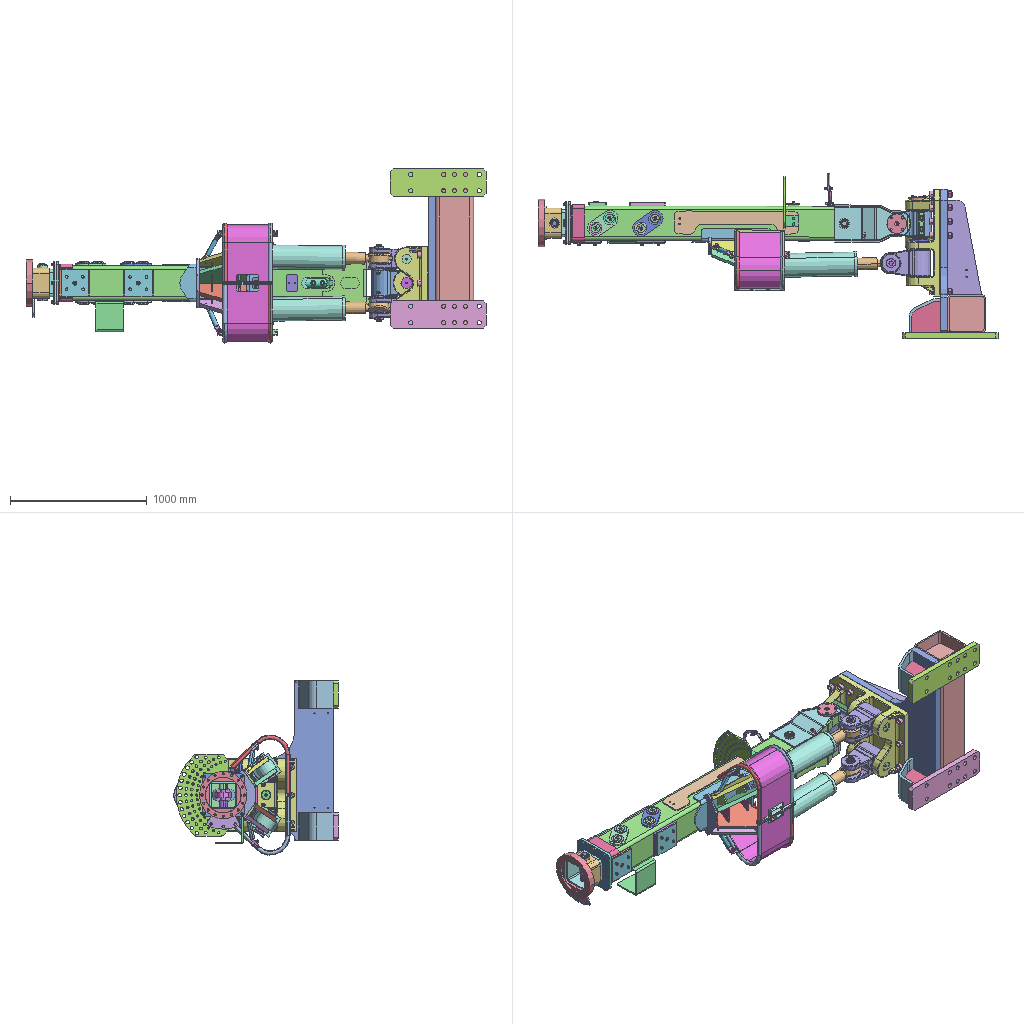Assembly | SolidWorks | 116 different items | 430 placed | box 3365 x 1207 x 1274 mm
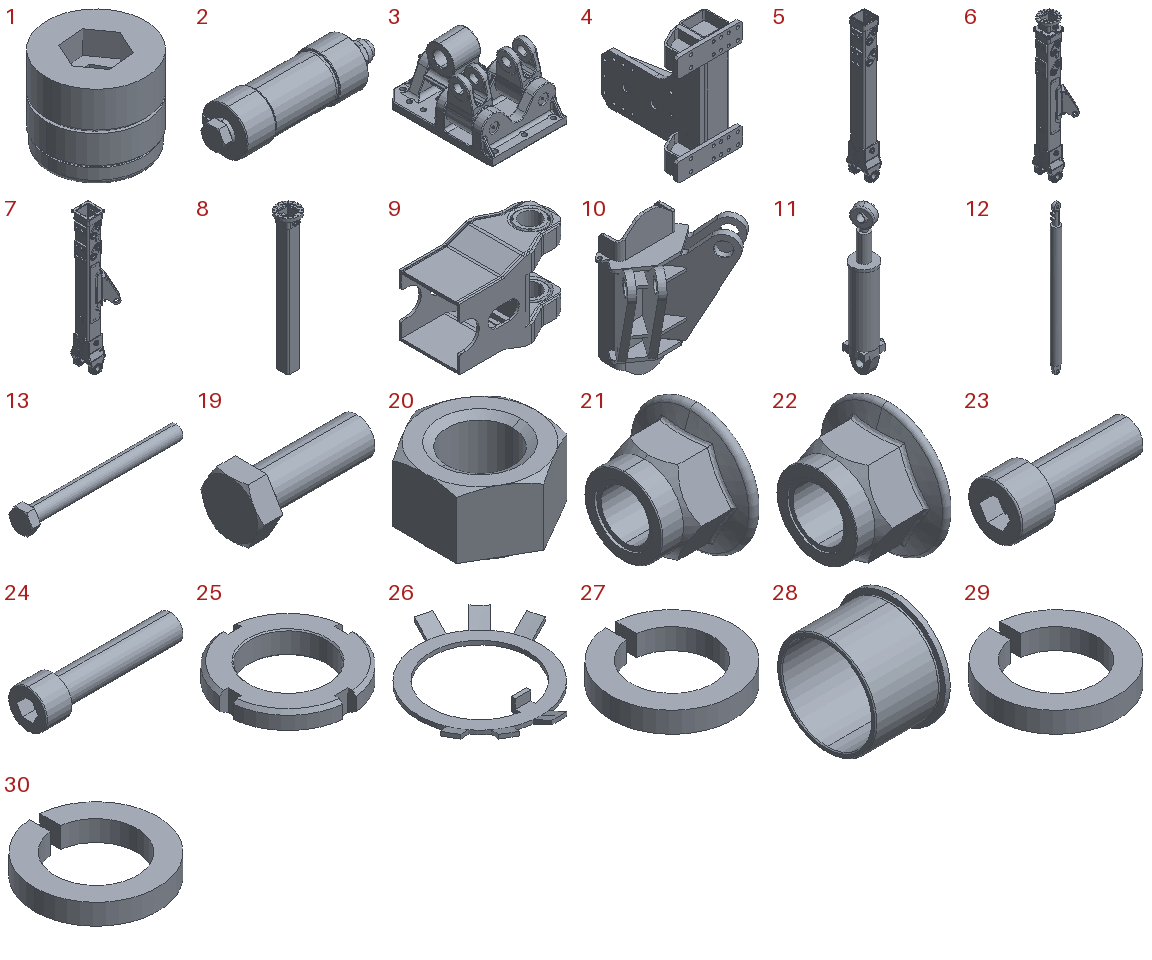Parts list (item | name | quantity | parent item | size | volume | features):
1 | (subassembly) | x14 | in 6 | 64 x 64 x 55 mm | 147055 mm3 | -
2 | (subassembly) | x4 | - | 222.5 x 65 x 65 mm | 514979 mm3 | features MirrorCompFeat 1, ReferencePattern 1
3 | (subassembly) | x1 | - | 533.36 x 780 x 459.48 mm | 60459444 mm3 | features CompositeCurve 2
4 | (subassembly) | x1 | - | 700 x 1090 x 1165 mm | 77907323 mm3 | features 3DProfileFeature 2, Cut 2, HoleWzd 2, MirrorCompFeat 2, ReferencePattern 2
5 | (subassembly) | x1 | in 7 | 291 x 352 x 2492 mm | 37081003 mm3 | features Cut 9, ReferencePattern 4, MirrorCompFeat 3, Chamfer 1, LocalLPattern 1, MirrorPattern 1, RefAxis 1
6 | (subassembly) | x1 | - | - | 96493183 mm3 | -
7 | (subassembly) | x1 | in 6 | 556.673 x 564.682 x 2503 mm | 53004232 mm3 | features MirrorCompFeat 3, ReferencePattern 3
8 | (subassembly) | x1 | in 6 | 348 x 348 x 2185 mm | 22246675 mm3 | features Cut 4, Chamfer 1, CosmeticWeldCutList 1
9 | (subassembly) | x1 | in 5 | 552.5 x 271 x 352 mm | 8203218 mm3 | features MirrorCompFeat 4, Cut 3, ReferencePattern 3, Chamfer 2, 3DProfileFeature 1, CirPattern 1, HoleWzd 1, MirrorPattern 1
10 | (subassembly) | x1 | in 7 | 564.682 x 359.673 x 650 mm | 12589036 mm3 | features ReferencePattern 8, MirrorCompFeat 6, Cut 2, Chamfer 1, LocalLPattern 1
11 | (subassembly) | x2 | - | 197.5 x 185 x 1126 mm | 10624377 mm3 | -
12 | (subassembly) | x1 | in 6 | 120 x 120 x 2210 mm | 15137402 mm3 | -
13 | - | x4 | in 2 | 222.5 x 34.641 x 30 mm | 75509 mm3 | features RevCut 3, Extrusion 1, Fillet 1, LPattern 1, Revolution 1
14 | - | x1 | in 9 | - | - | -
15 | - | x1 | in 9 | - | - | -
16 | - | x1 | in 9 | - | - | -
17 | - | x1 | in 9 | - | - | -
18 | - | x1 | in 9 | - | - | -
19 | - | x10 | in 6 | 42.5 x 20.785 x 18 mm | 6004 mm3 | features RevCut 3, Extrusion 1, Fillet 1, LPattern 1, Revolution 1
20 | - | x11 | - | 44.037 x 50.85 x 25.6 mm | 28405 mm3 | features ICE 2, RevCut 2, Extrusion 1
21 | - | x10 | - | 16.1 x 26 x 26 mm | 3234 mm3 | features Cut 2, Revolution 2, Boss 1, Chamfer 1, Fillet 1
22 | - | x4 | in 2 | 24.8 x 42.8 x 42.8 mm | 13100 mm3 | features Cut 2, Revolution 2, Boss 1, Chamfer 1, Fillet 1
23 | - | x6 | in 3 | 40 x 16 x 16 mm | 4080 mm3 | features BlendCut 1, Cut 1, Fillet 1, LPattern 1, RevCut 1, Revolution 1
24 | - | x12 | - | 170 x 45 x 45 mm | 138762 mm3 | features BlendCut 1, Cut 1, Fillet 1, LPattern 1, RevCut 1, Revolution 1
25 | - | x2 | in 6 | 54.672 x 54.672 x 10 mm | 12577 mm3 | features Chamfer 3, CirPattern 1, Cut 1, Extrusion 1
26 | - | x2 | in 6 | 56.873 x 59.449 x 5 mm | 1338 mm3 | features Boss 1, Cut 1, Revolution 1
27 | - | x8 | - | 15.372 x 15.344 x 2.6 mm | 261.313 mm3 | features Extrusion 1
28 | - | x4 | in 3 | 70 x 110 x 110 mm | 112148 mm3 | features Revolution 1
29 | - | x46 | in 3, 6 | 18.367 x 18.334 x 3.1 mm | 444.091 mm3 | features Extrusion 1
30 | - | x4 | - | 24.356 x 24.313 x 4.1 mm | 1031 mm3 | features Extrusion 1
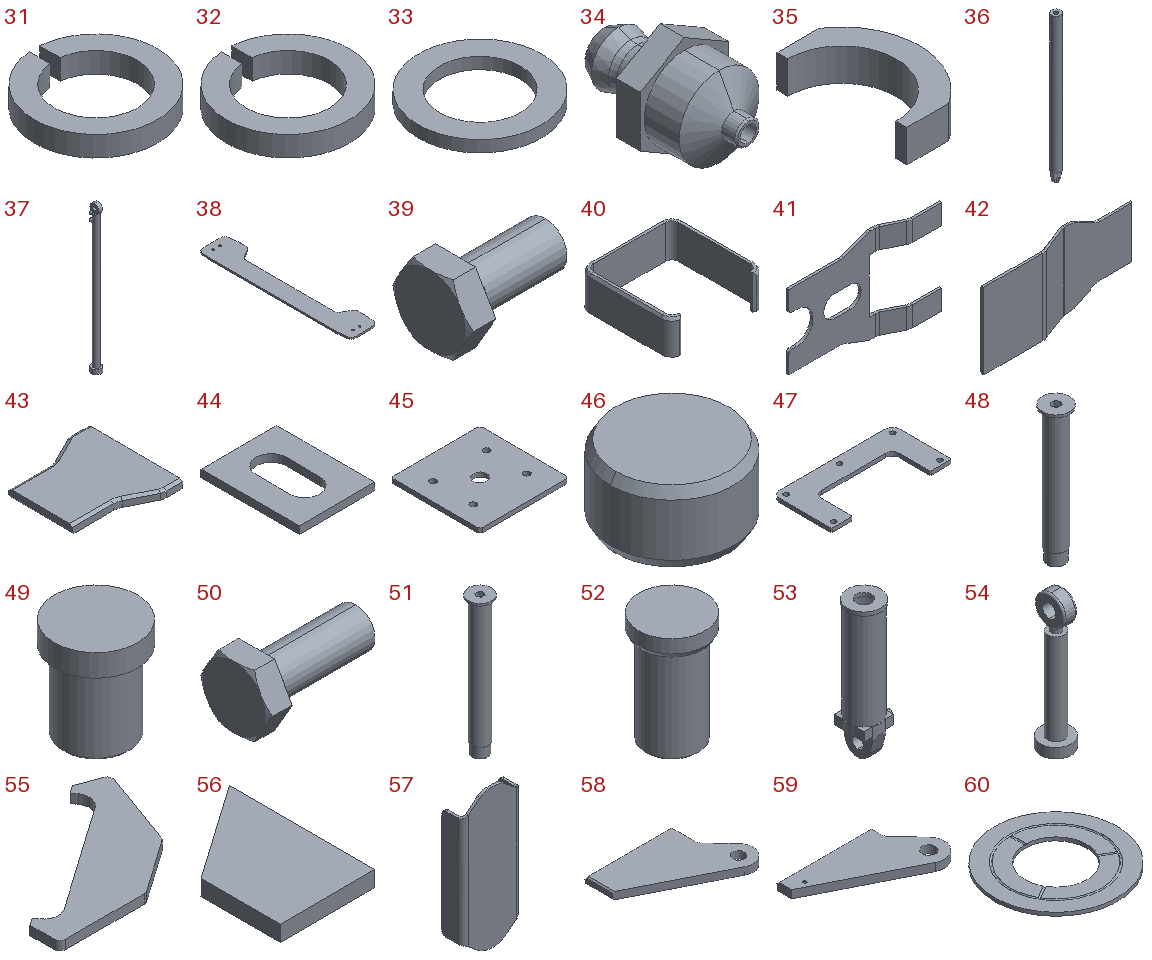31 | - | x4 | in 2 | 30.149 x 30.097 x 5 mm | 1905 mm3 | features Extrusion 1
32 | - | x11 | - | 45.424 x 45.346 x 7.5 mm | 6464 mm3 | features Extrusion 1
33 | - | x4 | in 3 | 16 x 16 x 1.5 mm | 171.708 mm3 | features Extrusion 1
34 | - | x20 | in 1, 3, 6 | 11 x 18 x 12.702 mm | 898.201 mm3 | features Boss 1, Chamfer 1, Revolution 1
35 | - | x2 | in 9 | 100 x 168 x 42 mm | 287014 mm3 | features ICE 2, Extrusion 1
36 | - | x1 | in 12 | 120 x 120 x 1920 mm | 9594518 mm3 | features ICE 4, Extrusion 1
37 | - | x1 | in 12 | 100 x 110 x 1610 mm | 5542883 mm3 | features ICE 5, Fillet 2, Extrusion 1
38 | - | x2 | in 7 | 170 x 909.794 x 10 mm | 1088199 mm3 | features 3DProfileFeature 1, Extrusion 1, HoleWzd 1
39 | - | x4 | in 3 | 26.4 x 18.475 x 16 mm | 2959 mm3 | features RevCut 3, Extrusion 1, Fillet 1, LPattern 1, Revolution 1
40 | - | x1 | in 5 | 276 x 274.941 x 100 mm | 939173 mm3 | features Chamfer 2, Extrusion 1, FlatPattern 1, RefAxis 1, SheetMetal 1, SolidToSheetMetal 1
41 | - | x2 | in 9 | 530 x 51.056 x 352 mm | 1033403 mm3 | features Fillet 3, Cut 1, Extrusion 1, FlatPattern 1, ICE 1, SheetMetal 1, SolidToSheetMetal 1
42 | - | x2 | in 9 | 530 x 50 x 251 mm | 1438713 mm3 | features Chamfer 2, Cut 1, Extrusion 1, FlatPattern 1, SheetMetal 1, SolidToSheetMetal 1
43 | - | x2 | in 9 | 250 x 251 x 20 mm | 983303 mm3 | features Chamfer 2, Extrusion 1
44 | - | x1 | in 9 | 202 x 261 x 20 mm | 809909 mm3 | features Cut 1, Extrusion 1
45 | - | x2 | in 6 | 200 x 200 x 10 mm | 386274 mm3 | features Chamfer 1, Extrusion 1, ICE 1
46 | - | x2 | in 9 | 130 x 130 x 75 mm | 972611 mm3 | features Chamfer 1, Extrusion 1
47 | - | x2 | in 6 | 310 x 152.5 x 10 mm | 269228 mm3 | features Chamfer 1, Extrusion 1, ICE 1
48 | - | x1 | in 6 | 55 x 55 x 275 mm | 342139 mm3 | features ICE 4, Chamfer 2, Fillet 2, Extrusion 1
49 | - | x2 | in 8 | 75 x 75 x 90 mm | 285538 mm3 | features Chamfer 1, Extrusion 1, ICE 1, RefAxis 1, RevCut 1
50 | - | x8 | - | 31.4 x 18.475 x 16 mm | 3352 mm3 | features RevCut 3, Extrusion 1, Fillet 1, LPattern 1, Revolution 1
51 | - | x1 | in 6 | 55 x 55 x 330 mm | 411254 mm3 | features ICE 4, Chamfer 2, Fillet 2, Extrusion 1
52 | - | x2 | in 5 | 75 x 75 x 125 mm | 382842 mm3 | features Chamfer 2, Extrusion 1, ICE 1, RefAxis 1, RevCut 1
53 | - | x2 | in 11 | 197.5 x 185 x 748 mm | 5801023 mm3 | features ICE 6, Extrusion 1
54 | - | x2 | in 11 | 155 x 155 x 685 mm | 4561292 mm3 | features ICE 3, Extrusion 1, Fillet 1, RevCut 1
55 | - | x2 | in 10 | 296.858 x 227.831 x 16 mm | 414208 mm3 | features Extrusion 1, Fillet 1
56 | - | x4 | in 10 | 72 x 110.415 x 12 mm | 73619 mm3 | features Extrusion 1
57 | - | x1 | in 10 | 274 x 100 x 650 mm | 2917891 mm3 | features Fillet 3, Extrusion 1, FlatPattern 1, ICE 1, SheetMetal 1, SolidToSheetMetal 1
58 | - | x1 | in 10 | 450 x 310 x 30 mm | 2452463 mm3 | features ICE 2, Chamfer 1, Extrusion 1, Fillet 1
59 | - | x1 | in 10 | 450 x 245.418 x 30 mm | 1807994 mm3 | features Chamfer 2, 3DProfileFeature 1, Extrusion 1, Fillet 1, HoleWzd 1, ICE 1
60 | - | x4 | in 3 | 180 x 180 x 5 mm | 93702 mm3 | features CirPattern 1, Extrusion 1, ICE 1, SweepCut 1
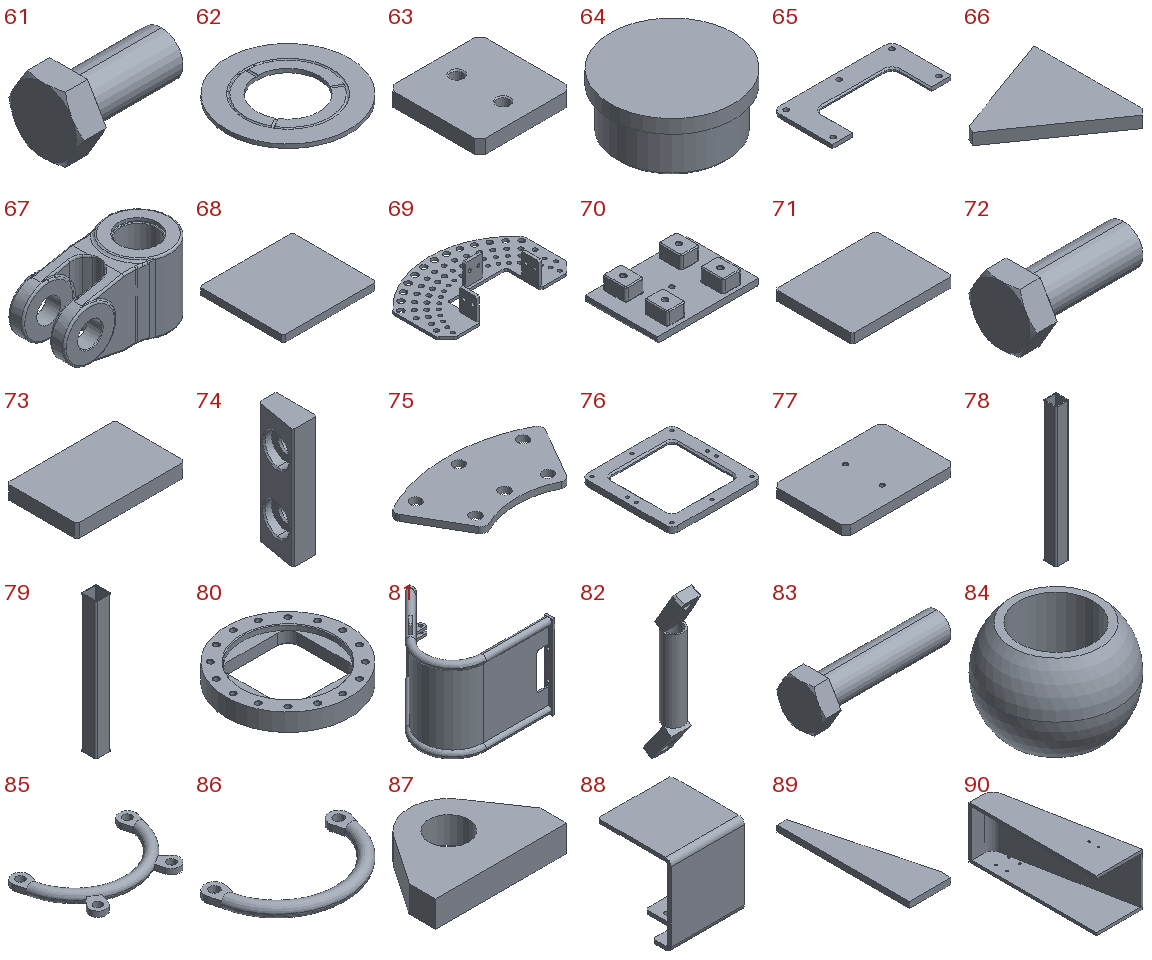61 | - | x10 | - | 32.5 x 20.785 x 18 mm | 4896 mm3 | features RevCut 3, Extrusion 1, Fillet 1, LPattern 1, Revolution 1
62 | - | x4 | in 3 | 160 x 160 x 5 mm | 73404 mm3 | features CirPattern 1, Extrusion 1, ICE 1, SweepCut 1
63 | - | x2 | in 7 | 80 x 80 x 12 mm | 74210 mm3 | features 3DProfileFeature 1, Chamfer 1, Extrusion 1, HoleWzd 1
64 | - | x8 | in 5 | 90 x 90 x 40 mm | 213919 mm3 | features Chamfer 1, Extrusion 1, ICE 1
65 | - | x2 | in 6 | 310 x 155 x 10 mm | 271244 mm3 | features Chamfer 2, Extrusion 1, ICE 1
66 | - | x2 | in 10 | 109.653 x 118.533 x 12 mm | 84519 mm3 | features Chamfer 1, Extrusion 1
67 | - | x2 | in 3 | 360 x 170 x 190 mm | 5382355 mm3 | features Fillet 14, ICE 11, Chamfer 4, MirrorPattern 2, Extrusion 1
68 | - | x2 | in 5 | 220 x 200 x 16 mm | 703200 mm3 | features Chamfer 1, Extrusion 1
69 | - | x1 | - | 600 x 380 x 112 mm | 1912190 mm3 | features ICE 7, Chamfer 4, Fillet 2, Extrusion 1
70 | - | x2 | in 6 | 220 x 156 x 41 mm | 648934 mm3 | features Fillet 4, ICE 3, 3DProfileFeature 2, HoleWzd 2, Chamfer 1, Extrusion 1
71 | - | x1 | in 5 | 260 x 200 x 25 mm | 1298750 mm3 | features Chamfer 1, Extrusion 1
72 | - | x8 | in 6 | 37.5 x 20.785 x 18 mm | 5461 mm3 | features RevCut 3, Extrusion 1, Fillet 1, LPattern 1, Revolution 1
73 | - | x1 | in 5 | 200 x 130 x 25 mm | 648750 mm3 | features Chamfer 1, Extrusion 1
74 | - | x2 | - | 31.677 x 55 x 160 mm | 198340 mm3 | features Chamfer 2, ICE 2, Extrusion 1
75 | - | x1 | - | 242.471 x 129.725 x 10 mm | 215713 mm3 | features Extrusion 1, Fillet 1, ICE 1
76 | - | x1 | in 7 | 310 x 310 x 20 mm | 773843 mm3 | features 3DProfileFeature 1, Chamfer 1, Extrusion 1, Fillet 1, HoleWzd 1, ICE 1
77 | - | x2 | in 7 | 120 x 80 x 10 mm | 95220 mm3 | features 3DProfileFeature 1, Chamfer 1, Extrusion 1, HoleWzd 1
78 | - | x1 | in 8 | 200 x 200 x 2150 mm | 18654812 mm3 | features Extrusion 1, Fillet 1, ICE 1
79 | - | x1 | in 5 | 250 x 250 x 2220 mm | 24230431 mm3 | features Chamfer 1, Extrusion 1, ICE 1, RefAxis 1
80 | - | x1 | in 8 | 348 x 348 x 50 mm | 2451722 mm3 | features Chamfer 2, ICE 2, 3DProfileFeature 1, CirPattern 1, Extrusion 1, HoleWzd 1
81 | - | x2 | - | 439 x 443.772 x 444 mm | 2517725 mm3 | features ICE 9, Chamfer 5, Sweep 2, BossThin 1
82 | - | x2 | - | 32 x 64.415 x 248.288 mm | 82986 mm3 | features ICE 4, Chamfer 2, Extrusion 1
83 | - | x18 | in 3 | 57.5 x 20.785 x 18 mm | 7723 mm3 | features RevCut 3, Extrusion 1, Fillet 1, LPattern 1, Revolution 1
84 | - | x2 | in 11 | 100 x 100 x 70 mm | 262061 mm3 | features ICE 2, Revolution 1
85 | - | x1 | - | 225.916 x 141.102 x 20 mm | 58505 mm3 | features ICE 3, MirrorPattern 1, Sweep 1
86 | - | x1 | - | 225.916 x 125 x 20 mm | 44773 mm3 | features ICE 2, MirrorPattern 1, Sweep 1
87 | - | x6 | in 7, 10 | 50 x 35 x 10 mm | 11273 mm3 | features Extrusion 1
88 | - | x1 | - | 200 x 200 x 220 mm | 944720 mm3 | features ICE 4, Fillet 3, Chamfer 1, Extrusion 1, FlatPattern 1, SheetMetal 1, SolidToSheetMetal 1
89 | - | x1 | in 4 | 210 x 670 x 30 mm | 2733000 mm3 | features Extrusion 1
90 | - | x1 | in 4 | 250 x 690 x 280 mm | 6785212 mm3 | features 3DProfileFeature 2, HoleWzd 2, ICE 2, Extrusion 1
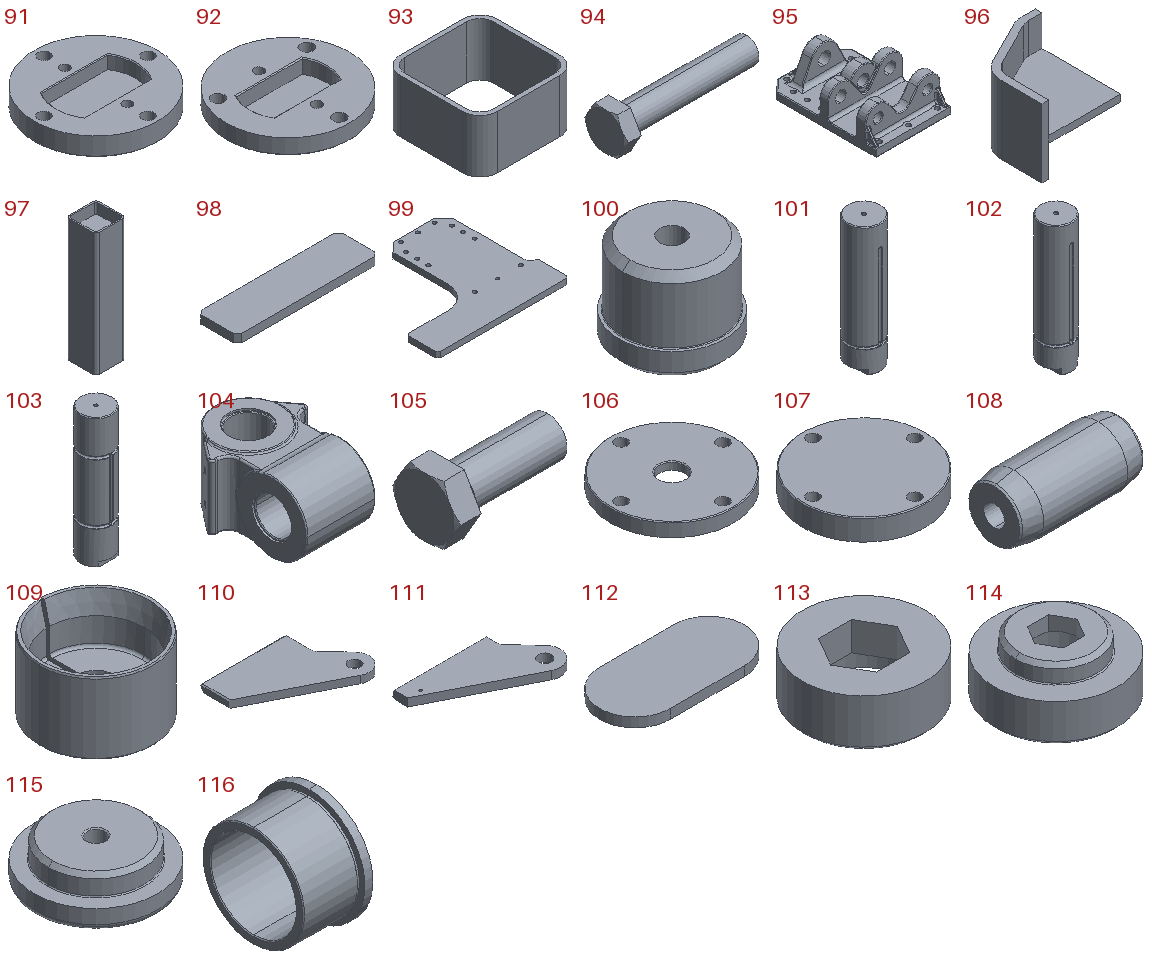91 | - | x1 | in 3 | 148 x 148 x 25 mm | 305929 mm3 | features Chamfer 3, ICE 3, 3DProfileFeature 1, Extrusion 1, HoleWzd 1
92 | - | x2 | in 3 | 138 x 138 x 20 mm | 204024 mm3 | features Chamfer 3, ICE 3, 3DProfileFeature 1, Extrusion 1, HoleWzd 1
93 | - | x1 | in 8 | 220 x 220 x 120 mm | 935894 mm3 | features Extrusion 1
94 | - | x2 | - | 67.5 x 20.785 x 18 mm | 8854 mm3 | features RevCut 3, Extrusion 1, Fillet 1, LPattern 1, Revolution 1
95 | - | x1 | in 3 | 530 x 780 x 260 mm | 33233633 mm3 | features Fillet 26, ICE 14, Chamfer 4, MirrorPattern 3, 3DProfileFeature 2, HoleWzd 2, LPattern 2, Extrusion 1
96 | - | x2 | in 4 | 230 x 250 x 200 mm | 2385457 mm3 | features Extrusion 1, ICE 1
97 | - | x1 | in 4 | 280 x 280 x 1165 mm | 17020849 mm3 | features ICE 2, Extrusion 1, MirrorPattern 1
98 | - | x2 | in 4 | 700 x 200 x 40 mm | 5568000 mm3 | features Chamfer 1, Extrusion 1
99 | - | x1 | in 4 | 1165 x 1050 x 50 mm | 36177793 mm3 | features Chamfer 3, ICE 2, 3DProfileFeature 1, Extrusion 1, HoleWzd 1
100 | - | x2 | in 3 | 75 x 75 x 63 mm | 232128 mm3 | features 3DProfileFeature 1, Chamfer 1, Extrusion 1, Fillet 1, HoleWzd 1, ICE 1
101 | - | x1 | in 3 | 90 x 90 x 350 mm | 2147115 mm3 | features Fillet 5, ICE 5, 3DProfileFeature 3, HoleWzd 3, Chamfer 2, RevCut 2, Extrusion 1, MirrorPattern 1, RefAxis 1
102 | - | x2 | in 3 | 80 x 80 x 330 mm | 1584103 mm3 | features ICE 5, Fillet 4, 3DProfileFeature 3, HoleWzd 3, Chamfer 2, RevCut 2, Extrusion 1, MirrorPattern 1, RefAxis 1
103 | - | x1 | - | 90 x 90 x 372 mm | 2295512 mm3 | features Fillet 5, ICE 5, 3DProfileFeature 2, HoleWzd 2, MirrorPattern 2, RevCut 2, Chamfer 1, Extrusion 1, RefAxis 1
104 | - | x1 | in 3 | 269.383 x 350 x 195 mm | 8603541 mm3 | features Fillet 12, ICE 10, MirrorPattern 3, Chamfer 2, 3DProfileFeature 1, Extrusion 1, HoleWzd 1
105 | - | x4 | - | 50 x 27.713 x 24 mm | 12952 mm3 | features RevCut 3, Extrusion 1, Fillet 1, LPattern 1, Revolution 1
106 | - | x1 | - | 145 x 145 x 16 mm | 201040 mm3 | features ICE 3, Chamfer 1, Extrusion 1
107 | - | x1 | - | 145 x 145 x 25 mm | 302931 mm3 | features Chamfer 2, ICE 2, Extrusion 1
108 | - | x4 | in 2 | 125 x 60 x 60 mm | 297103 mm3 | features 3DProfileFeature 1, Chamfer 1, HoleWzd 1, ICE 1, Revolution 1
109 | - | x8 | in 2 | 65 x 64.985 x 41.25 mm | 63691 mm3 | features Chamfer 2, ICE 2, 3DProfileFeature 1, Extrusion 1, Fillet 1, HoleWzd 1, RevCut 1
110 | - | x1 | in 10 | 450 x 310 x 30 mm | 2452463 mm3 | features MirrorStock 1
111 | - | x1 | in 10 | 450 x 245.418 x 30 mm | 1807994 mm3 | features MirrorStock 1
112 | - | x4 | in 5 | 245 x 120 x 16 mm | 420956 mm3 | features Extrusion 1
113 | - | x14 | in 1 | 64 x 64 x 25 mm | 53818 mm3 | features ICE 2, Chamfer 1, Extrusion 1
114 | - | x14 | in 1 | 64 x 64 x 29 mm | 46539 mm3 | features Chamfer 2, ICE 2, 3DProfileFeature 1, Extrusion 1, Fillet 1, HoleWzd 1
115 | - | x14 | in 1 | 62 x 62 x 20 mm | 45800 mm3 | features ICE 3, Fillet 2, 3DProfileFeature 1, Chamfer 1, Extrusion 1, HoleWzd 1
116 | - | x4 | in 3 | 60 x 105 x 105 mm | 135111 mm3 | features Revolution 1
Mates (type | each side: item.copy, entity, surface, feature), first 394 of 672 lines:
In the top assembly
Concentric | 103.1 face cylinder Boss-Extrude 1 | assembly face
Concentric | 103.1 face cylinder M10 Tapped Hole 1 | assembly face
Coincident | 103.1 face plane Boss-Extrude 1 | assembly face
Parallel | 103.1 face plane Cut-Extrude 4 | 107.1 face plane Cut-Extrude 2 | 2 times
Concentric | 103.1 face cylinder Boss-Extrude 1 | 60.1 face cylinder Boss-Extrude 1
Concentric | 103.1 face cylinder Boss-Extrude 1 | 60.2 face cylinder Boss-Extrude 1
Concentric | 28.1 face cylinder Revolve 1 | 103.1 face cylinder Boss-Extrude 1
Concentric | 103.1 face cylinder Boss-Extrude 1 | 106.1 face cylinder Boss-Extrude 1
Coincident | 99.1 face plane | 32.1 face plane Extrude 1
Coincident | 20.1 face plane Boss-Extrude 1 | 32.1 face plane Extrude 1
Concentric | 20.1 face cylinder Boss-Extrude 1 | 24.1 face cylinder Base-Revolve
Concentric | 32.1 face cylinder Extrude 1 | 24.1 face cylinder Base-Revolve
Coincident | 20.2 face plane Boss-Extrude 1 | 32.2 face plane Extrude 1
Concentric | 24.2 face cylinder Base-Revolve | 20.2 face cylinder Boss-Extrude 1
Concentric | 24.2 face cylinder Base-Revolve | 32.2 face cylinder Extrude 1
Coincident | 99.1 face plane | 32.2 face plane Extrude 1
Coincident | 20.3 face plane Boss-Extrude 1 | 32.3 face plane Extrude 1
Concentric | 24.3 face cylinder Base-Revolve | 20.3 face cylinder Boss-Extrude 1
Concentric | 24.3 face cylinder Base-Revolve | 32.3 face cylinder Extrude 1
Coincident | 99.1 face plane | 32.3 face plane Extrude 1
Coincident | 20.4 face plane Boss-Extrude 1 | 32.4 face plane Extrude 1
Concentric | 24.4 face cylinder Base-Revolve | 20.4 face cylinder Boss-Extrude 1
Concentric | 24.4 face cylinder Base-Revolve | 32.4 face cylinder Extrude 1
Coincident | 99.1 face plane | 32.4 face plane Extrude 1
Coincident | 20.5 face plane Boss-Extrude 1 | 32.5 face plane Extrude 1
Concentric | 24.5 face cylinder Base-Revolve | 20.5 face cylinder Boss-Extrude 1
Concentric | 24.5 face cylinder Base-Revolve | 32.5 face cylinder Extrude 1
Coincident | 99.1 face plane | 32.5 face plane Extrude 1
Coincident | 20.6 face plane Boss-Extrude 1 | 32.6 face plane Extrude 1
Concentric | 24.6 face cylinder Base-Revolve | 20.6 face cylinder Boss-Extrude 1
Concentric | 24.6 face cylinder Base-Revolve | 32.6 face cylinder Extrude 1
Coincident | 99.1 face plane | 32.6 face plane Extrude 1
Coincident | 20.7 face plane Boss-Extrude 1 | 32.7 face plane Extrude 1
Concentric | 24.7 face cylinder Base-Revolve | 20.7 face cylinder Boss-Extrude 1
Concentric | 24.7 face cylinder Base-Revolve | 32.7 face cylinder Extrude 1
Coincident | 99.1 face plane | 32.7 face plane Extrude 1
Concentric | 107.1 face cylinder Cut-Extrude 1 | 27.1 face cylinder Extrude 1
Coincident | 107.1 face plane Boss-Extrude 1 | 27.1 face plane Extrude 1
Concentric | 50.1 face cylinder Boss-Revolve 1 | 27.1 face cylinder Extrude 1
Coincident | 50.1 face plane Base-Extrude | 27.1 face plane Extrude 1
Coincident | 103.1 face plane Boss-Extrude 1 | 107.1 face plane Cut-Extrude 2
Concentric | 103.1 face cylinder Boss-Extrude 1 | 107.1 face cylinder Boss-Extrude 1
Coincident | 81.1 face plane Boss-Extrude 5 | 81.2 face plane Boss-Extrude 5
Concentric | 81.1 face cylinder Cut-Extrude 5 | 81.2 face cylinder Cut-Extrude 5
Concentric | 81.2 face cylinder Boss-Extrude 6 | 82.1 face cylinder Cut-Extrude 2
Coincident | 81.2 face plane Boss-Extrude 6 | 82.1 face plane Boss-Extrude 3
Concentric | 85.1 face cylinder Boss-Extrude 1 | 86.1 face cylinder Boss-Extrude 1
Concentric | 85.1 face cylinder Mirror 1 | 86.1 face cylinder Mirror 1
Coincident | 85.1 face plane Mirror 1 | 86.1 face plane Mirror 1
Concentric | 81.1 face cylinder Boss-Extrude 6 | 82.2 face cylinder Cut-Extrude 2
Coincident | 81.1 face plane Boss-Extrude 6 | 82.2 face plane Boss-Extrude 3
Concentric | 105.1 face cylinder Boss-Revolve 1 | 30.1 face cylinder Extrude 1
Coincident | 105.1 face plane Base-Extrude | 30.1 face plane Extrude 1
Concentric | 74.1 face cylinder Cut-Extrude 3 | 105.1 face cylinder Boss-Revolve 1
Coincident | 74.1 face plane Cut-Extrude 2 | 30.1 face plane Extrude 1
Concentric | 105.2 face cylinder Boss-Revolve 1 | 30.2 face cylinder Extrude 1
Coincident | 105.2 face plane Base-Extrude | 30.2 face plane Extrude 1
Concentric | 74.1 face cylinder Cut-Extrude 3 | 105.2 face cylinder Boss-Revolve 1
Coincident | 74.1 face plane Cut-Extrude 2 | 30.2 face plane Extrude 1
Concentric | 105.3 face cylinder Boss-Revolve 1 | 30.3 face cylinder Extrude 1
Coincident | 105.3 face plane Base-Extrude | 30.3 face plane Extrude 1
Concentric | 74.2 face cylinder Cut-Extrude 3 | 105.3 face cylinder Boss-Revolve 1
Coincident | 74.2 face plane Cut-Extrude 2 | 30.3 face plane Extrude 1
Concentric | 105.4 face cylinder Boss-Revolve 1 | 30.4 face cylinder Extrude 1
Coincident | 105.4 face plane Base-Extrude | 30.4 face plane Extrude 1
Concentric | 74.2 face cylinder Cut-Extrude 3 | 105.4 face cylinder Boss-Revolve 1
Coincident | 74.2 face plane Cut-Extrude 2 | 30.4 face plane Extrude 1
Concentric | 50.2 face cylinder Boss-Revolve 1 | 27.2 face cylinder Extrude 1
Coincident | 50.2 face plane Base-Extrude | 27.2 face plane Extrude 1
Concentric | 107.1 face cylinder Cut-Extrude 1 | 27.2 face cylinder Extrude 1
Coincident | 107.1 face plane Boss-Extrude 1 | 27.2 face plane Extrude 1
Concentric | 50.3 face cylinder Boss-Revolve 1 | 27.3 face cylinder Extrude 1
Coincident | 50.3 face plane Base-Extrude | 27.3 face plane Extrude 1
Concentric | 107.1 face cylinder Cut-Extrude 1 | 27.3 face cylinder Extrude 1
Coincident | 107.1 face plane Boss-Extrude 1 | 27.3 face plane Extrude 1
Concentric | 50.4 face cylinder Boss-Revolve 1 | 27.4 face cylinder Extrude 1
Coincident | 50.4 face plane Base-Extrude | 27.4 face plane Extrude 1
Concentric | 107.1 face cylinder Cut-Extrude 1 | 27.4 face cylinder Extrude 1
Coincident | 107.1 face plane Boss-Extrude 1 | 27.4 face plane Extrude 1
Concentric | 50.5 face cylinder Boss-Revolve 1 | 27.5 face cylinder Extrude 1
Coincident | 50.5 face plane Base-Extrude | 27.5 face plane Extrude 1
Concentric | 106.1 face cylinder Cut-Extrude 1 | 27.5 face cylinder Extrude 1
Coincident | 106.1 face plane Boss-Extrude 1 | 27.5 face plane Extrude 1
Concentric | 50.6 face cylinder Boss-Revolve 1 | 27.6 face cylinder Extrude 1
Coincident | 50.6 face plane Base-Extrude | 27.6 face plane Extrude 1
Concentric | 106.1 face cylinder Cut-Extrude 1 | 27.6 face cylinder Extrude 1
Coincident | 106.1 face plane Boss-Extrude 1 | 27.6 face plane Extrude 1
Concentric | 50.7 face cylinder Boss-Revolve 1 | 27.7 face cylinder Extrude 1
Coincident | 50.7 face plane Base-Extrude | 27.7 face plane Extrude 1
Concentric | 106.1 face cylinder Cut-Extrude 1 | 27.7 face cylinder Extrude 1
Coincident | 106.1 face plane Boss-Extrude 1 | 27.7 face plane Extrude 1
Concentric | 50.8 face cylinder Boss-Revolve 1 | 27.8 face cylinder Extrude 1
Coincident | 50.8 face plane Base-Extrude | 27.8 face plane Extrude 1
Coincident | 106.1 face plane Boss-Extrude 1 | 27.8 face plane Extrude 1
Concentric | 106.1 face cylinder Cut-Extrude 1 | 50.8 face cylinder Boss-Revolve 1
Coincident | 103.1 face plane Cut-Extrude 7 | 33.1 face plane Extrude 1
Concentric | 103.1 face cylinder M10 Tapped Hole 2 | 33.1 face cylinder Extrude 1
Coincident | 39.1 face plane Base-Extrude | 33.1 face plane Extrude 1
Concentric | 103.1 face cylinder M10 Tapped Hole 2 | 39.1 face cylinder Boss-Revolve 1
Concentric | 103.1 face cylinder M10 Tapped Hole 1 | 34.1 face cylinder Revolve 2
Coincident | 103.1 face plane Boss-Extrude 1 | 34.1 face plane Revolve 2
Concentric | 83.1 face cylinder Boss-Revolve 1 | 21.1 face cylinder Cut-Extrude 3
Coincident | 85.1 face plane Boss-Extrude 2 | 21.1 face plane Base-Revolve
Concentric | 83.1 face cylinder Boss-Revolve 1 | 29.1 face cylinder Extrude 1
Coincident | 83.1 face plane Base-Extrude | 29.1 face plane Extrude 1
Concentric | 83.2 face cylinder Boss-Revolve 1 | 21.2 face cylinder Cut-Extrude 3
Concentric | 83.2 face cylinder Boss-Revolve 1 | 29.2 face cylinder Extrude 1
Coincident | 83.2 face plane Base-Extrude | 29.2 face plane Extrude 1
Concentric | 85.1 face cylinder Boss-Extrude 2 | 83.2 face cylinder Boss-Revolve 1
Coincident | 85.1 face plane Boss-Extrude 2 | 21.2 face plane Base-Revolve
Concentric | 83.3 face cylinder Boss-Revolve 1 | 21.3 face cylinder Cut-Extrude 3
Concentric | 83.3 face cylinder Boss-Revolve 1 | 29.3 face cylinder Extrude 1
Coincident | 83.3 face plane Base-Extrude | 29.3 face plane Extrude 1
Concentric | 85.1 face cylinder Mirror 1 | 83.3 face cylinder Boss-Revolve 1
Coincident | 86.1 face plane Mirror 1 | 21.3 face plane Base-Revolve
Coincident | 85.1 face plane Mirror 1 | 29.3 face plane Extrude 1
Concentric | 83.4 face cylinder Boss-Revolve 1 | 21.4 face cylinder Cut-Extrude 3
Concentric | 83.4 face cylinder Boss-Revolve 1 | 29.4 face cylinder Extrude 1
Coincident | 83.4 face plane Base-Extrude | 29.4 face plane Extrude 1
Concentric | 85.1 face cylinder Boss-Extrude 1 | 83.4 face cylinder Boss-Revolve 1
Coincident | 86.1 face plane Boss-Extrude 1 | 21.4 face plane Base-Revolve
Coincident | 85.1 face plane Boss-Extrude 1 | 29.4 face plane Extrude 1
Coincident | 81.2 face plane Boss-Extrude 5 | 21.5 face plane Base-Revolve
Concentric | 81.2 face cylinder Cut-Extrude 6 | 21.5 face cylinder Cut-Extrude 3
Concentric | 69.1 face cylinder Cut-Extrude 1 | 29.5 face cylinder Extrude 1
Concentric | 69.1 face cylinder Cut-Extrude 1 | 61.1 face cylinder Boss-Revolve 1
Coincident | 61.1 face plane Base-Extrude | 29.5 face plane Extrude 1
Coincident | 69.1 face plane Boss-Extrude 2 | 29.5 face plane Extrude 1
Coincident | 29.6 face plane Extrude 1 | 61.2 face plane Base-Extrude
Concentric | 69.1 face cylinder Cut-Extrude 1 | 29.6 face cylinder Extrude 1
Concentric | 69.1 face cylinder Cut-Extrude 1 | 61.2 face cylinder Boss-Revolve 1
Coincident | 69.1 face plane Boss-Extrude 2 | 29.6 face plane Extrude 1
Coincident | 29.7 face plane Extrude 1 | 61.3 face plane Base-Extrude
Concentric | 69.1 face cylinder Cut-Extrude 2 | 29.7 face cylinder Extrude 1
Concentric | 69.1 face cylinder Cut-Extrude 2 | 61.3 face cylinder Boss-Revolve 1
Coincident | 69.1 face plane Boss-Extrude 2 | 29.7 face plane Extrude 1
Coincident | 29.8 face plane Extrude 1 | 61.4 face plane Base-Extrude
Concentric | 69.1 face cylinder Cut-Extrude 2 | 29.8 face cylinder Extrude 1
Concentric | 69.1 face cylinder Cut-Extrude 2 | 61.4 face cylinder Boss-Revolve 1
Coincident | 69.1 face plane Boss-Extrude 2 | 29.8 face plane Extrude 1
Coincident | 29.9 face plane Extrude 1 | 61.5 face plane Base-Extrude
Concentric | 69.1 face cylinder Cut-Extrude 1 | 29.9 face cylinder Extrude 1
Coincident | 69.1 face plane Boss-Extrude 2 | 29.9 face plane Extrude 1
Concentric | 69.1 face cylinder Cut-Extrude 1 | 61.5 face cylinder Boss-Revolve 1
Coincident | 29.10 face plane Extrude 1 | 61.6 face plane Base-Extrude
Concentric | 69.1 face cylinder Cut-Extrude 1 | 29.10 face cylinder Extrude 1
Coincident | 69.1 face plane Boss-Extrude 2 | 29.10 face plane Extrude 1
Concentric | 69.1 face cylinder Cut-Extrude 1 | 61.6 face cylinder Boss-Revolve 1
Coincident | 61.7 face plane Base-Extrude | 29.11 face plane Extrude 1
Concentric | 88.1 face cylinder 转换Body 1 | 29.11 face cylinder Extrude 1
Coincident | 88.1 face plane 转换Body 1 | 29.11 face plane Extrude 1
Concentric | 88.1 face cylinder 转换Body 1 | 61.7 face cylinder Boss-Revolve 1
Coincident | 61.8 face plane Base-Extrude | 29.12 face plane Extrude 1
Concentric | 88.1 face cylinder 转换Body 1 | 29.12 face cylinder Extrude 1
Coincident | 88.1 face plane 转换Body 1 | 29.12 face plane Extrude 1
Concentric | 88.1 face cylinder 转换Body 1 | 61.8 face cylinder Boss-Revolve 1
Concentric | 81.2 face cylinder Cut-Extrude 6 | 94.1 face cylinder Boss-Revolve 1
Coincident | 81.2 face plane Boss-Extrude 5 | 94.1 face plane Base-Extrude
Coincident | 81.1 face plane Boss-Extrude 5 | 21.6 face plane Base-Revolve
Concentric | 81.1 face cylinder Cut-Extrude 6 | 21.6 face cylinder Cut-Extrude 3
Concentric | 81.1 face cylinder Cut-Extrude 6 | 94.2 face cylinder Boss-Revolve 1
Coincident | 81.1 face plane Boss-Extrude 5 | 94.2 face plane Base-Extrude
Concentric | 21.7 face cylinder Cut-Extrude 3 | 83.5 face cylinder Boss-Revolve 1
Concentric | 83.5 face cylinder Boss-Revolve 1 | 29.13 face cylinder Extrude 1
Coincident | 83.5 face plane Base-Extrude | 29.13 face plane Extrude 1
Concentric | 81.2 face cylinder Boss-Extrude 6 | 83.5 face cylinder Boss-Revolve 1
Coincident | 82.1 face plane Boss-Extrude 3 | 21.7 face plane Base-Revolve
Coincident | 81.2 face plane Boss-Extrude 6 | 29.13 face plane Extrude 1
Concentric | 21.8 face cylinder Cut-Extrude 3 | 83.6 face cylinder Boss-Revolve 1
Concentric | 83.6 face cylinder Boss-Revolve 1 | 29.14 face cylinder Extrude 1
Coincident | 83.6 face plane Base-Extrude | 29.14 face plane Extrude 1
Concentric | 81.1 face cylinder Boss-Extrude 6 | 83.6 face cylinder Boss-Revolve 1
Coincident | 82.2 face plane Boss-Extrude 3 | 21.8 face plane Base-Revolve
Coincident | 81.1 face plane Boss-Extrude 6 | 29.14 face plane Extrude 1
Coincident | 61.9 face plane Base-Extrude | 29.15 face plane Extrude 1
Concentric | 82.2 face cylinder Cut-Extrude 1 | 29.15 face cylinder Extrude 1
Coincident | 82.2 face plane Boss-Extrude 2 | 29.15 face plane Extrude 1
Concentric | 82.2 face cylinder Cut-Extrude 1 | 61.9 face cylinder Boss-Revolve 1
Coincident | 61.10 face plane Base-Extrude | 29.16 face plane Extrude 1
Concentric | 82.1 face cylinder Cut-Extrude 1 | 29.16 face cylinder Extrude 1
Coincident | 82.1 face plane Boss-Extrude 2 | 29.16 face plane Extrude 1
Concentric | 82.1 face cylinder Cut-Extrude 1 | 61.10 face cylinder Boss-Revolve 1
Concentric | 83.7 face cylinder Boss-Revolve 1 | 21.9 face cylinder Cut-Extrude 3
Concentric | 83.7 face cylinder Boss-Revolve 1 | 29.17 face cylinder Extrude 1
Coincident | 83.7 face plane Base-Extrude | 29.17 face plane Extrude 1
Concentric | 81.1 face cylinder Cut-Extrude 5 | 83.7 face cylinder Boss-Revolve 1
Coincident | 81.1 face plane Boss-Extrude 4 | 21.9 face plane Base-Revolve
Coincident | 81.2 face plane Boss-Extrude 4 | 29.17 face plane Extrude 1
Concentric | 83.8 face cylinder Boss-Revolve 1 | 21.10 face cylinder Cut-Extrude 3
Concentric | 83.8 face cylinder Boss-Revolve 1 | 29.18 face cylinder Extrude 1
Coincident | 83.8 face plane Base-Extrude | 29.18 face plane Extrude 1
Concentric | 81.1 face cylinder Cut-Extrude 5 | 83.8 face cylinder Boss-Revolve 1
Coincident | 81.1 face plane Boss-Extrude 4 | 21.10 face plane Base-Revolve
Coincident | 81.2 face plane Boss-Extrude 4 | 29.18 face plane Extrude 1
Coincident | 99.1 face plane | 95.1 face plane Boss-Extrude 1
Concentric | 95.1 face cylinder Cut-Extrude 1 | 32.1 face cylinder Extrude 1
Coincident | 95.1 face plane Boss-Extrude 1 | 24.1 face plane Base-Revolve
Concentric | 95.1 face cylinder Cut-Extrude 1 | 32.2 face cylinder Extrude 1
Coincident | 95.1 face plane Boss-Extrude 1 | 24.2 face plane Base-Revolve
Coincident | 95.1 face plane Boss-Extrude 1 | 24.3 face plane Base-Revolve
Concentric | 95.1 face cylinder Cut-Extrude 1 | 32.3 face cylinder Extrude 1
Coincident | 95.1 face plane Boss-Extrude 1 | 24.4 face plane Base-Revolve
Concentric | 95.1 face cylinder Cut-Extrude 1 | 32.4 face cylinder Extrude 1
Coincident | 95.1 face plane Boss-Extrude 1 | 24.5 face plane Base-Revolve
Concentric | 95.1 face cylinder Cut-Extrude 1 | 32.5 face cylinder Extrude 1
Coincident | 95.1 face plane Boss-Extrude 1 | 24.6 face plane Base-Revolve
Concentric | 95.1 face cylinder Cut-Extrude 1 | 32.6 face cylinder Extrude 1
Coincident | 95.1 face plane Boss-Extrude 1 | 24.7 face plane Base-Revolve
Concentric | 95.1 face cylinder Cut-Extrude 1 | 32.7 face cylinder Extrude 1
Concentric | 95.1 face cylinder Cut-Extrude 1 | 24.8 face cylinder Base-Revolve
Coincident | 95.1 face plane Boss-Extrude 1 | 24.8 face plane Base-Revolve
Concentric | 99.1 face cylinder | 95.1 face cylinder Cut-Extrude 1 | 2 times
Concentric | 104.1 face cylinder Cut-Extrude 1 | 28.1 face cylinder Revolve 1
Coincident | 104.1 face plane Cut-Extrude 5 | 28.1 face plane Revolve 1
Concentric | 104.1 face cylinder Cut-Extrude 1 | 28.2 face cylinder Revolve 1
Coincident | 104.1 face plane Cut-Extrude 4 | 28.2 face plane Revolve 1
Coincident | 104.1 face plane Boss-Extrude 1 | 60.2 face plane Boss-Extrude 1
Coincident | 104.1 face plane Boss-Extrude 1 | 60.1 face plane Boss-Extrude 1
Concentric | 104.1 face cylinder M16 Tapped Hole 1 | 105.4 face cylinder Boss-Revolve 1
Concentric | 104.1 face cylinder M16 Tapped Hole 1 | 105.3 face cylinder Boss-Revolve 1
Coincident | 104.1 face plane Boss-Extrude 1 | 74.2 face plane Boss-Extrude 1
Concentric | 104.1 face cylinder Mirror 3 | 105.1 face cylinder Boss-Revolve 1
Concentric | 104.1 face cylinder Mirror 3 | 105.2 face cylinder Boss-Revolve 1
Coincident | 104.1 face plane Boss-Extrude 1 | 74.1 face plane Boss-Extrude 1
Coincident | 80.1 face plane Boss-Extrude 1 | 75.1 face plane Boss-Extrude 1
Concentric | 80.1 face cylinder Boss-Extrude 1 | 75.1 face cylinder Boss-Extrude 1
Concentric | 80.1 face cylinder CirPattern 1 | 75.1 face cylinder Boss-Extrude 1
Concentric | 103.1 face cylinder Boss-Extrude 1 | 46.1 face cylinder Cut-Extrude 2
Coincident | 107.1 face plane Boss-Extrude 1 | 42.1 face plane
Coincident | 106.1 face plane Boss-Extrude 1 | 42.2 face plane
Concentric | 63.1 face cylinder M12 Tapped Hole 1 | 88.1 face cylinder 转换Body 1
Concentric | 63.1 edge | 88.1 face cylinder 转换Body 1
Coincident | 63.1 face plane Boss-Extrude 1 | 88.1 face plane 转换Body 1
Tangent | 59.1 edge | 82.1 face plane Cut-Extrude 1
Concentric | 63.2 face cylinder M12 Tapped Hole 1 | 69.1 face cylinder Cut-Extrude 2 | 2 times
Coincident | 63.2 face plane Boss-Extrude 1 | 69.1 face plane Boss-Extrude 2
Concentric | 87.1 face cylinder Boss-Extrude 1 | 85.1 face cylinder Boss-Extrude 2
Concentric | 87.2 face cylinder Boss-Extrude 1 | 85.1 face cylinder Boss-Extrude 2
Coincident | 87.2 face plane Boss-Extrude 1 | 85.1 face plane Boss-Extrude 2
Concentric | 87.3 face cylinder Boss-Extrude 1 | 81.1 face cylinder Cut-Extrude 6
Coincident | 87.3 face plane Boss-Extrude 1 | 81.1 face plane Boss-Extrude 5
Concentric | 87.4 face cylinder Boss-Extrude 1 | 81.2 face cylinder Cut-Extrude 6
Concentric | 46.2 face cylinder M12 Tapped Hole 1 | 107.1 face cylinder Cut-Extrude 1
Concentric | 46.1 face cylinder Mirror 1 | 27.8 face cylinder Extrude 1
Concentric | 87.2 face cylinder Boss-Extrude 1 | 83.1 face cylinder Boss-Revolve 1
Coincident | 87.2 face plane Boss-Extrude 1 | 29.1 face plane Extrude 1
Coincident | 87.1 face plane Boss-Extrude 1 | 29.2 face plane Extrude 1
Width | 43.1 face plane | 43.2 face plane | 60.1 face plane Boss-Extrude 1 | 60.2 face plane Boss-Extrude 1
Width | 84.1 face plane Cut-Extrude 2 | 84.1 face plane Cut-Extrude 2 | 67.1 face plane Cut-Extrude 1 | 67.1 face plane Cut-Extrude 1
Concentric | 53.1 face cylinder Boss-Extrude 3 | 58.1 face cylinder Cut-Extrude 1
Width | 53.1 face plane Boss-Extrude 3 | 53.1 face plane Boss-Extrude 3 | 59.1 face plane | 58.1 face plane
Width | 84.2 face plane Cut-Extrude 2 | 84.2 face plane Cut-Extrude 2 | 67.2 face plane Cut-Extrude 1 | 67.2 face plane Cut-Extrude 1
Width | 53.2 face plane Boss-Extrude 3 | 53.2 face plane Boss-Extrude 3 | 110.1 face plane | 111.1 face plane
Concentric | 53.2 face cylinder Boss-Extrude 3 | 110.1 face cylinder Cut-Extrude 2
Concentric | 67.1 face cylinder Cut-Extrude 2 | 108.1 face cylinder Revolve 1
Width | 109.1 face plane Boss-Extrude 1 | 109.2 face plane Boss-Extrude 1 | 67.1 face plane Boss-Extrude 1 | 67.1 face plane Boss-Extrude 1
Concentric | 84.1 face cylinder Cut-Extrude 1 | 108.1 face cylinder Revolve 1
Concentric | 67.2 face cylinder Cut-Extrude 2 | 108.2 face cylinder Revolve 1
Width | 109.3 face plane Boss-Extrude 1 | 109.4 face plane Boss-Extrude 1 | 67.2 face plane Boss-Extrude 1 | 67.2 face plane Boss-Extrude 1
Concentric | 84.2 face cylinder Cut-Extrude 1 | 108.2 face cylinder Revolve 1
Concentric | 59.1 face cylinder Cut-Extrude 1 | 108.3 face cylinder Revolve 1
Width | 109.5 face plane Boss-Extrude 1 | 109.6 face plane Boss-Extrude 1 | 58.1 face plane | 59.1 face plane
Concentric | 53.1 face cylinder Boss-Extrude 3 | 108.3 face cylinder Revolve 1
Concentric | 110.1 face cylinder Cut-Extrude 2 | 108.4 face cylinder Revolve 1
Width | 109.7 face plane Boss-Extrude 1 | 109.8 face plane Boss-Extrude 1 | 111.1 face plane | 110.1 face plane
In subassembly 3
Concentric | 95.2 face cylinder LPattern 1 | 3.1 face
Coincident | 95.2 face | 3.1 face | 3 times
Concentric | 95.2 face cylinder LPattern 2 | 3.1 face | 2 times
Coincident | 95.2 face plane Boss-Extrude 2 | 91.1 face plane Boss-Extrude 1
Concentric | 95.2 face cylinder M12 Tapped Hole 1 | 91.1 face cylinder Cut-Extrude 6
Coincident | 95.2 face plane Boss-Extrude 5 | 92.1 face plane Boss-Extrude 1
Concentric | 95.2 face cylinder M12 Tapped Hole 2 | 92.1 face cylinder Cut-Extrude 6
Concentric | 95.2 face cylinder LPattern 2 | 102.1 face cylinder Boss-Extrude 1
Coincident | 95.2 face plane Cut-Extrude 10 | 102.1 face plane Boss-Extrude 1
Coincident | 95.2 face plane Cut-Extrude 10 | 102.2 face plane Boss-Extrude 1
Concentric | 95.2 face cylinder Cut-Extrude 10 | 102.2 face cylinder Boss-Extrude 1
Concentric | 95.2 face cylinder Cut-Extrude 9 | 101.1 face cylinder Boss-Extrude 1
Coincident | 95.2 face plane Cut-Extrude 9 | 101.1 face plane Boss-Extrude 1
Concentric | 101.1 face cylinder Boss-Extrude 1 | 91.1 face cylinder Boss-Extrude 1
Concentric | 102.2 face cylinder Boss-Extrude 1 | 92.2 face cylinder Boss-Extrude 1
Parallel | 102.2 face plane Cut-Extrude 14 | 92.2 face plane Cut-Extrude 1
Concentric | 95.2 face cylinder M12 Tapped Hole 2 | 92.2 face cylinder Cut-Extrude 6
Coincident | 95.2 face plane Mirror 2 | 92.2 face plane Boss-Extrude 1
Concentric | 102.1 face cylinder Boss-Extrude 1 | 92.1 face cylinder Boss-Extrude 1
Concentric | 101.1 face cylinder M10 Tapped Hole 1 | 34.1 face cylinder Revolve 2
Coincident | 101.1 face plane Boss-Extrude 1 | 34.1 face plane Revolve 2
Concentric | 102.1 face cylinder M10x1.0 Tapped Hole 1 | 34.2 face cylinder Revolve 2
Coincident | 102.1 face plane Boss-Extrude 1 | 34.2 face plane Revolve 2
Concentric | 102.2 face cylinder M10x1.0 Tapped Hole 1 | 34.3 face cylinder Revolve 2
Coincident | 102.2 face plane Boss-Extrude 1 | 34.3 face plane Revolve 2
Concentric | 101.1 face cylinder M10 Tapped Hole 2 | 39.1 face cylinder Boss-Revolve 1
Concentric | 83.1 face cylinder Boss-Revolve 1 | 29.1 face cylinder Extrude 1
Coincident | 83.1 face plane Base-Extrude | 29.1 face plane Extrude 1
Concentric | 91.1 face cylinder Cut-Extrude 6 | 83.1 face cylinder Boss-Revolve 1
Coincident | 91.1 face plane Cut-Extrude 3 | 29.1 face plane Extrude 1
Concentric | 83.2 face cylinder Boss-Revolve 1 | 29.2 face cylinder Extrude 1
Coincident | 83.2 face plane Base-Extrude | 29.2 face plane Extrude 1
Concentric | 91.1 face cylinder Cut-Extrude 6 | 83.2 face cylinder Boss-Revolve 1
Coincident | 91.1 face plane Cut-Extrude 3 | 29.2 face plane Extrude 1
Concentric | 83.3 face cylinder Boss-Revolve 1 | 29.3 face cylinder Extrude 1
Coincident | 83.3 face plane Base-Extrude | 29.3 face plane Extrude 1
Concentric | 91.1 face cylinder Cut-Extrude 6 | 83.3 face cylinder Boss-Revolve 1
Coincident | 91.1 face plane Cut-Extrude 3 | 29.3 face plane Extrude 1
Concentric | 83.4 face cylinder Boss-Revolve 1 | 29.4 face cylinder Extrude 1
Coincident | 83.4 face plane Base-Extrude | 29.4 face plane Extrude 1
Concentric | 91.1 face cylinder Cut-Extrude 6 | 83.4 face cylinder Boss-Revolve 1
Coincident | 91.1 face plane Cut-Extrude 3 | 29.4 face plane Extrude 1
Concentric | 83.9 face cylinder Boss-Revolve 1 | 29.6 face cylinder Extrude 1
Coincident | 83.9 face plane Base-Extrude | 29.6 face plane Extrude 1
Concentric | 92.1 face cylinder Cut-Extrude 6 | 83.9 face cylinder Boss-Revolve 1
Coincident | 92.1 face plane Cut-Extrude 3 | 29.6 face plane Extrude 1
Concentric | 83.10 face cylinder Boss-Revolve 1 | 29.7 face cylinder Extrude 1
Coincident | 83.10 face plane Base-Extrude | 29.7 face plane Extrude 1
Concentric | 92.1 face cylinder Cut-Extrude 6 | 83.10 face cylinder Boss-Revolve 1
Coincident | 92.1 face plane Cut-Extrude 3 | 29.7 face plane Extrude 1
Concentric | 83.11 face cylinder Boss-Revolve 1 | 29.8 face cylinder Extrude 1
Coincident | 83.11 face plane Base-Extrude | 29.8 face plane Extrude 1
Concentric | 92.1 face cylinder Cut-Extrude 6 | 83.11 face cylinder Boss-Revolve 1
Coincident | 92.1 face plane Cut-Extrude 3 | 29.8 face plane Extrude 1
Concentric | 83.12 face cylinder Boss-Revolve 1 | 29.19 face cylinder Extrude 1
Coincident | 83.12 face plane Base-Extrude | 29.19 face plane Extrude 1
Concentric | 92.2 face cylinder Cut-Extrude 6 | 83.12 face cylinder Boss-Revolve 1
Coincident | 92.2 face plane Cut-Extrude 3 | 29.19 face plane Extrude 1
Concentric | 83.13 face cylinder Boss-Revolve 1 | 29.9 face cylinder Extrude 1
Coincident | 83.13 face plane Base-Extrude | 29.9 face plane Extrude 1
Concentric | 92.2 face cylinder Cut-Extrude 6 | 83.13 face cylinder Boss-Revolve 1
Coincident | 92.2 face plane Cut-Extrude 3 | 29.9 face plane Extrude 1
Concentric | 83.14 face cylinder Boss-Revolve 1 | 29.10 face cylinder Extrude 1
Coincident | 83.14 face plane Base-Extrude | 29.10 face plane Extrude 1
Concentric | 92.2 face cylinder Cut-Extrude 6 | 83.14 face cylinder Boss-Revolve 1
Coincident | 92.2 face plane Cut-Extrude 3 | 29.10 face plane Extrude 1
Concentric | 92.2 face cylinder 打Hole尺寸(%根据)内六角圆柱头Screw的类型1 | 23.1 face cylinder Base-Revolve
Coincident | 92.2 face plane 打Hole尺寸(%根据)内六角圆柱头Screw的类型1 | 23.1 face plane Base-Revolve
Concentric | 92.2 face cylinder 打Hole尺寸(%根据)内六角圆柱头Screw的类型1 | 23.2 face cylinder Base-Revolve
Coincident | 92.2 face plane 打Hole尺寸(%根据)内六角圆柱头Screw的类型1 | 23.2 face plane Base-Revolve
Concentric | 91.1 face cylinder 打Hole尺寸(%根据)内六角圆柱头Screw的类型1 | 23.3 face cylinder Base-Revolve
Coincident | 91.1 face plane 打Hole尺寸(%根据)内六角圆柱头Screw的类型1 | 23.3 face plane Base-Revolve
Concentric | 91.1 face cylinder 打Hole尺寸(%根据)内六角圆柱头Screw的类型1 | 23.4 face cylinder Base-Revolve
Coincident | 91.1 face plane 打Hole尺寸(%根据)内六角圆柱头Screw的类型1 | 23.4 face plane Base-Revolve
Concentric | 92.1 face cylinder 打Hole尺寸(%根据)内六角圆柱头Screw的类型1 | 23.5 face cylinder Base-Revolve
Coincident | 92.1 face plane 打Hole尺寸(%根据)内六角圆柱头Screw的类型1 | 23.5 face plane Base-Revolve
Concentric | 92.1 face cylinder 打Hole尺寸(%根据)内六角圆柱头Screw的类型1 | 23.6 face cylinder Base-Revolve
Coincident | 92.1 face plane 打Hole尺寸(%根据)内六角圆柱头Screw的类型1 | 23.6 face plane Base-Revolve
Concentric | 102.1 face cylinder M10 Tapped Hole 4 | 39.2 face cylinder Boss-Revolve 1
Concentric | 102.2 face cylinder M10 Tapped Hole 4 | 39.3 face cylinder Boss-Revolve 1
Concentric | 95.2 face cylinder Cut-Extrude 2 | 100.1 face cylinder Boss-Extrude 1
Coincident | 95.2 face plane Boss-Extrude 1 | 100.1 face plane Boss-Extrude 2
Concentric | 95.2 face cylinder Cut-Extrude 2 | 100.2 face cylinder Boss-Extrude 1
Coincident | 95.2 face plane Boss-Extrude 1 | 100.2 face plane Boss-Extrude 2
Concentric | 39.1 face cylinder Boss-Revolve 1 | 33.1 face cylinder Extrude 1
Coincident | 39.1 face plane Base-Extrude | 33.1 face plane Extrude 1
Coincident | 101.1 face plane Cut-Extrude 10 | 33.1 edge
Concentric | 39.2 face cylinder Boss-Revolve 1 | 33.2 face cylinder Extrude 1
Coincident | 39.2 face plane Base-Extrude | 33.2 face plane Extrude 1
Coincident | 102.1 face plane Cut-Extrude 13 | 33.2 face plane Extrude 1
Concentric | 39.3 face cylinder Boss-Revolve 1 | 33.3 face cylinder Extrude 1
Coincident | 39.3 face plane Base-Extrude | 33.3 face plane Extrude 1
Coincident | 102.2 face plane Cut-Extrude 13 | 33.3 face plane Extrude 1
Concentric | 104.2 edge | 28.3 face cylinder Revolve 1
Concentric | 60.3 face cylinder Boss-Extrude 1 | 28.3 face cylinder Revolve 1
Coincident | 104.2 face plane Cut-Extrude 2 | 28.3 face plane Revolve 1
Coincident | 104.2 face plane Boss-Extrude 1 | 60.3 face plane Boss-Extrude 1
Concentric | 28.4 face cylinder Revolve 1 | 60.4 face cylinder Boss-Extrude 1
Concentric | 104.2 face cylinder Boss-Extrude 1 | 28.4 face cylinder Revolve 1
Coincident | 104.2 face plane Cut-Extrude 3 | 28.4 face plane Revolve 1
Coincident | 104.2 face plane Boss-Extrude 1 | 60.4 face plane Boss-Extrude 1
Concentric | 101.1 face cylinder Boss-Extrude 1 | 28.3 face cylinder Revolve 1
Width | 95.2 face plane Boss-Extrude 7 | 95.2 face plane Boss-Extrude 2 | 104.2 face plane Cut-Extrude 10 | 104.2 face plane Mirror 2
Concentric | 116.1 face cylinder Revolve 1 | 67.3 face cylinder Boss-Extrude 1
Coincident | 116.1 face plane Revolve 1 | 67.3 face plane Cut-Extrude 4
Concentric | 116.1 face cylinder Revolve 1 | 62.1 face cylinder Boss-Extrude 1
Coincident | 62.1 face plane Boss-Extrude 1 | 67.3 face plane Boss-Extrude 1
Concentric | 67.3 face cylinder Boss-Extrude 1 | 116.2 face cylinder Revolve 1
Coincident | 67.3 face plane Cut-Extrude 3 | 116.2 face plane Revolve 1
Concentric | 116.2 face cylinder Revolve 1 | 62.2 face cylinder Boss-Extrude 1
Coincident | 67.3 face plane Boss-Extrude 1 | 62.2 face plane Boss-Extrude 1
Concentric | 102.1 face cylinder Boss-Extrude 1 | 116.1 face cylinder Revolve 1
Width | 67.3 face plane Mirror 4 | 67.3 face plane Cut-Extrude 11 | 95.2 face plane Boss-Extrude 5 | 95.2 face plane Boss-Extrude 8
Concentric | 116.3 face cylinder Revolve 1 | 67.4 face cylinder Boss-Extrude 1
Coincident | 116.3 face plane Revolve 1 | 67.4 face plane Cut-Extrude 4
Concentric | 116.3 face cylinder Revolve 1 | 62.3 face cylinder Boss-Extrude 1
Coincident | 62.3 face plane Boss-Extrude 1 | 67.4 face plane Boss-Extrude 1
Concentric | 116.4 face cylinder Revolve 1 | 67.4 face cylinder Boss-Extrude 1
Coincident | 116.4 face plane Revolve 1 | 67.4 face plane Cut-Extrude 3
Concentric | 116.4 face cylinder Revolve 1 | 62.4 face cylinder Boss-Extrude 1
Coincident | 62.4 face plane Boss-Extrude 1 | 67.4 face plane Boss-Extrude 1
Concentric | 102.2 face cylinder Boss-Extrude 1 | 116.3 face cylinder Revolve 1
Width | 67.4 face plane Mirror 4 | 67.4 face plane Cut-Extrude 11 | 95.2 face plane Boss-Extrude 5 | 95.2 face plane Boss-Extrude 8
In subassembly 4
Coincident | 97.1 face plane | 99.2 face plane | 2 times
Width | 99.2 face plane | 99.2 face plane | 97.1 face plane | 97.1 face plane
Coincident | 97.1 face plane | 98.1 face plane | 2 times